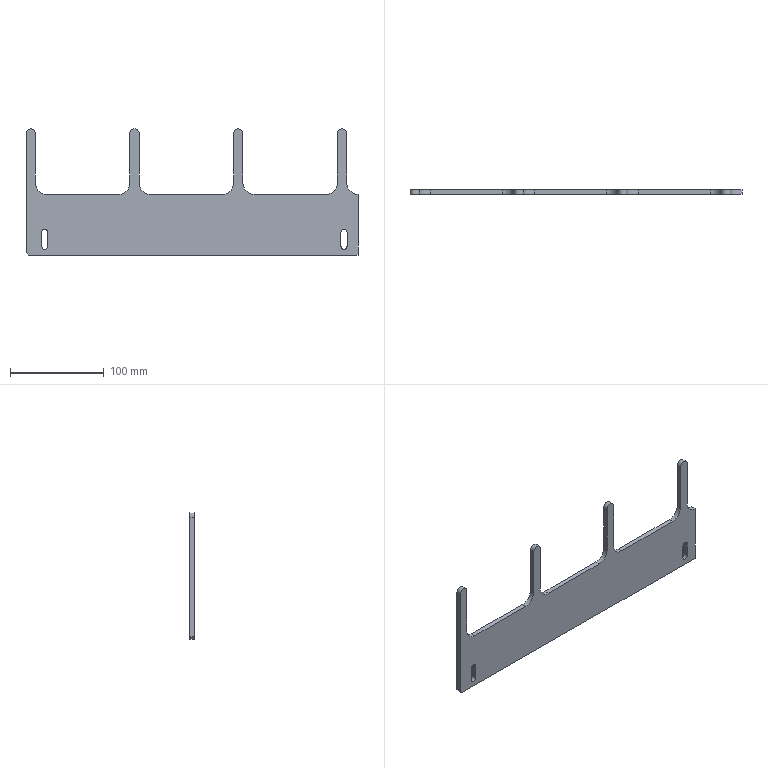Part | SolidWorks | features BaseBody 1, ICE 1 | 1 solid | 35 faces | box 355 x 5 x 135 mm | volume 128920 mm3 | plane 20 | cylinder 15 | commonest cylinder face diameters 24 x7 6.5 x4 10 x4
STEP:
#1=CARTESIAN_POINT('',(-205.,0.,-5.));
#2=VERTEX_POINT('',#1);
#3=CARTESIAN_POINT('',(-205.,0.,60.));
#4=VERTEX_POINT('',#3);
#5=CARTESIAN_POINT('',(-205.,0.,62.5));
#6=DIRECTION('',(0.,0.,1.));
#7=VECTOR('',#6,1000.);
#8=LINE('',#5,#7);
#9=EDGE_CURVE('',#2,#4,#8,.T.);
#10=ORIENTED_EDGE('',*,*,#9,.F.);
#11=CARTESIAN_POINT('',(-557.5,0.,-5.));
#12=VERTEX_POINT('',#11);
#13=CARTESIAN_POINT('',(-557.5,0.,-5.));
#14=DIRECTION('',(1.,0.,0.));
#15=VECTOR('',#14,1000.);
#16=LINE('',#13,#15);
#17=EDGE_CURVE('',#12,#2,#16,.T.);
#18=ORIENTED_EDGE('',*,*,#17,.F.);
#19=CARTESIAN_POINT('',(-560.,0.,-2.5));
#20=VERTEX_POINT('',#19);
#21=CARTESIAN_POINT('',(-560.,0.,-2.5));
#22=DIRECTION('',(0.7071,0.,-0.7071));
#23=VECTOR('',#22,1000.);
#24=LINE('',#21,#23);
#25=EDGE_CURVE('',#20,#12,#24,.T.);
#26=ORIENTED_EDGE('',*,*,#25,.F.);
#27=CARTESIAN_POINT('',(-560.,0.,125.));
#28=VERTEX_POINT('',#27);
#29=CARTESIAN_POINT('',(-560.,0.,125.));
#30=DIRECTION('',(0.,0.,-1.));
#31=VECTOR('',#30,1000.);
#32=LINE('',#29,#31);
#33=EDGE_CURVE('',#28,#20,#32,.T.);
#34=ORIENTED_EDGE('',*,*,#33,.F.);
#35=CARTESIAN_POINT('',(-550.,0.,125.));
#36=VERTEX_POINT('',#35);
#37=CARTESIAN_POINT('',(-555.,0.,125.));
#38=DIRECTION('',(0.,-1.,0.));
#39=DIRECTION('',(1.,0.,0.));
#40=AXIS2_PLACEMENT_3D('',#37,#38,#39);
#41=CIRCLE('',#40,5.);
#42=EDGE_CURVE('',#36,#28,#41,.T.);
#43=ORIENTED_EDGE('',*,*,#42,.F.);
#44=CARTESIAN_POINT('',(-550.,0.,72.));
#45=VERTEX_POINT('',#44);
#46=CARTESIAN_POINT('',(-550.,0.,72.));
#47=DIRECTION('',(0.,0.,1.));
#48=VECTOR('',#47,1000.);
#49=LINE('',#46,#48);
#50=EDGE_CURVE('',#45,#36,#49,.T.);
#51=ORIENTED_EDGE('',*,*,#50,.F.);
#52=CARTESIAN_POINT('',(-538.,0.,60.));
#53=VERTEX_POINT('',#52);
#54=CARTESIAN_POINT('',(-538.,0.,72.));
#55=DIRECTION('',(0.,1.,0.));
#56=DIRECTION('',(0.,0.,-1.));
#57=AXIS2_PLACEMENT_3D('',#54,#55,#56);
#58=CIRCLE('',#57,12.);
#59=EDGE_CURVE('',#53,#45,#58,.T.);
#60=ORIENTED_EDGE('',*,*,#59,.F.);
#61=CARTESIAN_POINT('',(-461.,0.,60.));
#62=VERTEX_POINT('',#61);
#63=CARTESIAN_POINT('',(-461.,0.,60.));
#64=DIRECTION('',(-1.,0.,0.));
#65=VECTOR('',#64,1000.);
#66=LINE('',#63,#65);
#67=EDGE_CURVE('',#62,#53,#66,.T.);
#68=ORIENTED_EDGE('',*,*,#67,.F.);
#69=CARTESIAN_POINT('',(-449.,0.,72.));
#70=VERTEX_POINT('',#69);
#71=CARTESIAN_POINT('',(-461.,0.,72.));
#72=DIRECTION('',(0.,1.,0.));
#73=DIRECTION('',(1.,0.,0.));
#74=AXIS2_PLACEMENT_3D('',#71,#72,#73);
#75=CIRCLE('',#74,12.);
#76=EDGE_CURVE('',#70,#62,#75,.T.);
#77=ORIENTED_EDGE('',*,*,#76,.F.);
#78=CARTESIAN_POINT('',(-449.,0.,125.));
#79=VERTEX_POINT('',#78);
#80=CARTESIAN_POINT('',(-449.,0.,125.));
#81=DIRECTION('',(0.,0.,-1.));
#82=VECTOR('',#81,1000.);
#83=LINE('',#80,#82);
#84=EDGE_CURVE('',#79,#70,#83,.T.);
#85=ORIENTED_EDGE('',*,*,#84,.F.);
#86=CARTESIAN_POINT('',(-439.,0.,125.));
#87=VERTEX_POINT('',#86);
#88=CARTESIAN_POINT('',(-444.,0.,125.));
#89=DIRECTION('',(0.,-1.,0.));
#90=DIRECTION('',(1.,0.,0.));
#91=AXIS2_PLACEMENT_3D('',#88,#89,#90);
#92=CIRCLE('',#91,5.);
#93=EDGE_CURVE('',#87,#79,#92,.T.);
#94=ORIENTED_EDGE('',*,*,#93,.F.);
#95=CARTESIAN_POINT('',(-439.,0.,72.));
#96=VERTEX_POINT('',#95);
#97=CARTESIAN_POINT('',(-439.,0.,72.));
#98=DIRECTION('',(0.,0.,1.));
#99=VECTOR('',#98,1000.);
#100=LINE('',#97,#99);
#101=EDGE_CURVE('',#96,#87,#100,.T.);
#102=ORIENTED_EDGE('',*,*,#101,.F.);
#103=CARTESIAN_POINT('',(-427.,0.,60.));
#104=VERTEX_POINT('',#103);
#105=CARTESIAN_POINT('',(-427.,0.,72.));
#106=DIRECTION('',(0.,1.,0.));
#107=DIRECTION('',(0.,0.,-1.));
#108=AXIS2_PLACEMENT_3D('',#105,#106,#107);
#109=CIRCLE('',#108,12.);
#110=EDGE_CURVE('',#104,#96,#109,.T.);
#111=ORIENTED_EDGE('',*,*,#110,.F.);
#112=CARTESIAN_POINT('',(-350.,0.,60.));
#113=VERTEX_POINT('',#112);
#114=CARTESIAN_POINT('',(-350.,0.,60.));
#115=DIRECTION('',(-1.,0.,0.));
#116=VECTOR('',#115,1000.);
#117=LINE('',#114,#116);
#118=EDGE_CURVE('',#113,#104,#117,.T.);
#119=ORIENTED_EDGE('',*,*,#118,.F.);
#120=CARTESIAN_POINT('',(-338.,0.,72.));
#121=VERTEX_POINT('',#120);
#122=CARTESIAN_POINT('',(-350.,0.,72.));
#123=DIRECTION('',(0.,1.,0.));
#124=DIRECTION('',(1.,0.,0.));
#125=AXIS2_PLACEMENT_3D('',#122,#123,#124);
#126=CIRCLE('',#125,12.);
#127=EDGE_CURVE('',#121,#113,#126,.T.);
#128=ORIENTED_EDGE('',*,*,#127,.F.);
#129=CARTESIAN_POINT('',(-338.,0.,125.));
#130=VERTEX_POINT('',#129);
#131=CARTESIAN_POINT('',(-338.,0.,125.));
#132=DIRECTION('',(0.,0.,-1.));
#133=VECTOR('',#132,1000.);
#134=LINE('',#131,#133);
#135=EDGE_CURVE('',#130,#121,#134,.T.);
#136=ORIENTED_EDGE('',*,*,#135,.F.);
#137=CARTESIAN_POINT('',(-328.,0.,125.));
#138=VERTEX_POINT('',#137);
#139=CARTESIAN_POINT('',(-333.,0.,125.));
#140=DIRECTION('',(0.,-1.,0.));
#141=DIRECTION('',(1.,0.,0.));
#142=AXIS2_PLACEMENT_3D('',#139,#140,#141);
#143=CIRCLE('',#142,5.);
#144=EDGE_CURVE('',#138,#130,#143,.T.);
#145=ORIENTED_EDGE('',*,*,#144,.F.);
#146=CARTESIAN_POINT('',(-328.,0.,72.));
#147=VERTEX_POINT('',#146);
#148=CARTESIAN_POINT('',(-328.,0.,72.));
#149=DIRECTION('',(0.,0.,1.));
#150=VECTOR('',#149,1000.);
#151=LINE('',#148,#150);
#152=EDGE_CURVE('',#147,#138,#151,.T.);
#153=ORIENTED_EDGE('',*,*,#152,.F.);
#154=CARTESIAN_POINT('',(-316.,0.,60.));
#155=VERTEX_POINT('',#154);
#156=CARTESIAN_POINT('',(-316.,0.,72.));
#157=DIRECTION('',(0.,1.,0.));
#158=DIRECTION('',(0.,0.,-1.));
#159=AXIS2_PLACEMENT_3D('',#156,#157,#158);
#160=CIRCLE('',#159,12.);
#161=EDGE_CURVE('',#155,#147,#160,.T.);
#162=ORIENTED_EDGE('',*,*,#161,.F.);
#163=CARTESIAN_POINT('',(-239.,0.,60.));
#164=VERTEX_POINT('',#163);
#165=CARTESIAN_POINT('',(-239.,0.,60.));
#166=DIRECTION('',(-1.,0.,0.));
#167=VECTOR('',#166,1000.);
#168=LINE('',#165,#167);
#169=EDGE_CURVE('',#164,#155,#168,.T.);
#170=ORIENTED_EDGE('',*,*,#169,.F.);
#171=CARTESIAN_POINT('',(-227.,0.,72.));
#172=VERTEX_POINT('',#171);
#173=CARTESIAN_POINT('',(-239.,0.,72.));
#174=DIRECTION('',(0.,1.,0.));
#175=DIRECTION('',(1.,0.,0.));
#176=AXIS2_PLACEMENT_3D('',#173,#174,#175);
#177=CIRCLE('',#176,12.);
#178=EDGE_CURVE('',#172,#164,#177,.T.);
#179=ORIENTED_EDGE('',*,*,#178,.F.);
#180=CARTESIAN_POINT('',(-227.,0.,125.));
#181=VERTEX_POINT('',#180);
#182=CARTESIAN_POINT('',(-227.,0.,125.));
#183=DIRECTION('',(0.,0.,-1.));
#184=VECTOR('',#183,1000.);
#185=LINE('',#182,#184);
#186=EDGE_CURVE('',#181,#172,#185,.T.);
#187=ORIENTED_EDGE('',*,*,#186,.F.);
#188=CARTESIAN_POINT('',(-217.,0.,125.));
#189=VERTEX_POINT('',#188);
#190=CARTESIAN_POINT('',(-222.,0.,125.));
#191=DIRECTION('',(0.,-1.,0.));
#192=DIRECTION('',(1.,0.,0.));
#193=AXIS2_PLACEMENT_3D('',#190,#191,#192);
#194=CIRCLE('',#193,5.);
#195=EDGE_CURVE('',#189,#181,#194,.T.);
#196=ORIENTED_EDGE('',*,*,#195,.F.);
#197=CARTESIAN_POINT('',(-217.,0.,72.));
#198=VERTEX_POINT('',#197);
#199=CARTESIAN_POINT('',(-217.,0.,72.));
#200=DIRECTION('',(0.,0.,1.));
#201=VECTOR('',#200,1000.);
#202=LINE('',#199,#201);
#203=EDGE_CURVE('',#198,#189,#202,.T.);
#204=ORIENTED_EDGE('',*,*,#203,.F.);
#205=CARTESIAN_POINT('',(-205.,0.,72.));
#206=DIRECTION('',(0.,1.,0.));
#207=DIRECTION('',(0.,0.,-1.));
#208=AXIS2_PLACEMENT_3D('',#205,#206,#207);
#209=CIRCLE('',#208,12.);
#210=EDGE_CURVE('',#4,#198,#209,.T.);
#211=ORIENTED_EDGE('',*,*,#210,.F.);
#212=EDGE_LOOP('',(#10,#18,#26,#34,#43,#51,#60,#68,#77,#85,#94,#102,#111,#119,#128,#136,#145,#153,#162,#170,#179,#187,#196,#204,#211));
#213=FACE_OUTER_BOUND('',#212,.T.);
#214=CARTESIAN_POINT('',(-536.75,0.,4.5));
#215=VERTEX_POINT('',#214);
#216=CARTESIAN_POINT('',(-543.25,0.,4.5));
#217=VERTEX_POINT('',#216);
#218=CARTESIAN_POINT('',(-540.,0.,4.5));
#219=DIRECTION('',(0.,1.,0.));
#220=DIRECTION('',(1.,0.,0.));
#221=AXIS2_PLACEMENT_3D('',#218,#219,#220);
#222=CIRCLE('',#221,3.25);
#223=EDGE_CURVE('',#215,#217,#222,.T.);
#224=ORIENTED_EDGE('',*,*,#223,.F.);
#225=CARTESIAN_POINT('',(-536.75,0.,19.5));
#226=VERTEX_POINT('',#225);
#227=CARTESIAN_POINT('',(-536.75,0.,19.5));
#228=DIRECTION('',(0.,0.,-1.));
#229=VECTOR('',#228,1000.);
#230=LINE('',#227,#229);
#231=EDGE_CURVE('',#226,#215,#230,.T.);
#232=ORIENTED_EDGE('',*,*,#231,.F.);
#233=CARTESIAN_POINT('',(-543.25,0.,19.5));
#234=VERTEX_POINT('',#233);
#235=CARTESIAN_POINT('',(-540.,0.,19.5));
#236=DIRECTION('',(0.,1.,0.));
#237=DIRECTION('',(-1.,0.,0.));
#238=AXIS2_PLACEMENT_3D('',#235,#236,#237);
#239=CIRCLE('',#238,3.25);
#240=EDGE_CURVE('',#234,#226,#239,.T.);
#241=ORIENTED_EDGE('',*,*,#240,.F.);
#242=CARTESIAN_POINT('',(-543.25,0.,4.5));
#243=DIRECTION('',(0.,0.,1.));
#244=VECTOR('',#243,1000.);
#245=LINE('',#242,#244);
#246=EDGE_CURVE('',#217,#234,#245,.T.);
#247=ORIENTED_EDGE('',*,*,#246,.F.);
#248=EDGE_LOOP('',(#224,#232,#241,#247));
#249=FACE_BOUND('',#248,.T.);
#250=CARTESIAN_POINT('',(-216.75,0.,4.5));
#251=VERTEX_POINT('',#250);
#252=CARTESIAN_POINT('',(-223.25,0.,4.5));
#253=VERTEX_POINT('',#252);
#254=CARTESIAN_POINT('',(-220.,0.,4.5));
#255=DIRECTION('',(0.,1.,0.));
#256=DIRECTION('',(1.,0.,0.));
#257=AXIS2_PLACEMENT_3D('',#254,#255,#256);
#258=CIRCLE('',#257,3.25);
#259=EDGE_CURVE('',#251,#253,#258,.T.);
#260=ORIENTED_EDGE('',*,*,#259,.F.);
#261=CARTESIAN_POINT('',(-216.75,0.,19.5));
#262=VERTEX_POINT('',#261);
#263=CARTESIAN_POINT('',(-216.75,0.,19.5));
#264=DIRECTION('',(0.,0.,-1.));
#265=VECTOR('',#264,1000.);
#266=LINE('',#263,#265);
#267=EDGE_CURVE('',#262,#251,#266,.T.);
#268=ORIENTED_EDGE('',*,*,#267,.F.);
#269=CARTESIAN_POINT('',(-223.25,0.,19.5));
#270=VERTEX_POINT('',#269);
#271=CARTESIAN_POINT('',(-220.,0.,19.5));
#272=DIRECTION('',(0.,1.,0.));
#273=DIRECTION('',(-1.,0.,0.));
#274=AXIS2_PLACEMENT_3D('',#271,#272,#273);
#275=CIRCLE('',#274,3.25);
#276=EDGE_CURVE('',#270,#262,#275,.T.);
#277=ORIENTED_EDGE('',*,*,#276,.F.);
#278=CARTESIAN_POINT('',(-223.25,0.,4.5));
#279=DIRECTION('',(0.,0.,1.));
#280=VECTOR('',#279,1000.);
#281=LINE('',#278,#280);
#282=EDGE_CURVE('',#253,#270,#281,.T.);
#283=ORIENTED_EDGE('',*,*,#282,.F.);
#284=EDGE_LOOP('',(#260,#268,#277,#283));
#285=FACE_BOUND('',#284,.T.);
#286=CARTESIAN_POINT('',(0.,0.,62.5));
#287=DIRECTION('',(0.,1.,0.));
#288=DIRECTION('',(0.,0.,-1.));
#289=AXIS2_PLACEMENT_3D('',#286,#287,#288);
#290=PLANE('',#289);
#291=ADVANCED_FACE('',(#213,#249,#285),#290,.T.);
#292=CARTESIAN_POINT('',(-205.,-5.,60.));
#293=VERTEX_POINT('',#292);
#294=CARTESIAN_POINT('',(-205.,-5.,-5.));
#295=VERTEX_POINT('',#294);
#296=CARTESIAN_POINT('',(-205.,-5.,60.));
#297=DIRECTION('',(0.,0.,-1.));
#298=VECTOR('',#297,1000.);
#299=LINE('',#296,#298);
#300=EDGE_CURVE('',#293,#295,#299,.T.);
#301=ORIENTED_EDGE('',*,*,#300,.F.);
#302=CARTESIAN_POINT('',(-217.,-5.,72.));
#303=VERTEX_POINT('',#302);
#304=CARTESIAN_POINT('',(-205.,-5.,72.));
#305=DIRECTION('',(0.,-1.,0.));
#306=DIRECTION('',(-1.,0.,0.));
#307=AXIS2_PLACEMENT_3D('',#304,#305,#306);
#308=CIRCLE('',#307,12.);
#309=EDGE_CURVE('',#303,#293,#308,.T.);
#310=ORIENTED_EDGE('',*,*,#309,.F.);
#311=CARTESIAN_POINT('',(-217.,-5.,125.));
#312=VERTEX_POINT('',#311);
#313=CARTESIAN_POINT('',(-217.,-5.,125.));
#314=DIRECTION('',(0.,0.,-1.));
#315=VECTOR('',#314,1000.);
#316=LINE('',#313,#315);
#317=EDGE_CURVE('',#312,#303,#316,.T.);
#318=ORIENTED_EDGE('',*,*,#317,.F.);
#319=CARTESIAN_POINT('',(-227.,-5.,125.));
#320=VERTEX_POINT('',#319);
#321=CARTESIAN_POINT('',(-222.,-5.,125.));
#322=DIRECTION('',(0.,1.,0.));
#323=DIRECTION('',(-1.,0.,0.));
#324=AXIS2_PLACEMENT_3D('',#321,#322,#323);
#325=CIRCLE('',#324,5.);
#326=EDGE_CURVE('',#320,#312,#325,.T.);
#327=ORIENTED_EDGE('',*,*,#326,.F.);
#328=CARTESIAN_POINT('',(-227.,-5.,72.));
#329=VERTEX_POINT('',#328);
#330=CARTESIAN_POINT('',(-227.,-5.,72.));
#331=DIRECTION('',(0.,0.,1.));
#332=VECTOR('',#331,1000.);
#333=LINE('',#330,#332);
#334=EDGE_CURVE('',#329,#320,#333,.T.);
#335=ORIENTED_EDGE('',*,*,#334,.F.);
#336=CARTESIAN_POINT('',(-239.,-5.,60.));
#337=VERTEX_POINT('',#336);
#338=CARTESIAN_POINT('',(-239.,-5.,72.));
#339=DIRECTION('',(0.,-1.,0.));
#340=DIRECTION('',(0.,0.,-1.));
#341=AXIS2_PLACEMENT_3D('',#338,#339,#340);
#342=CIRCLE('',#341,12.);
#343=EDGE_CURVE('',#337,#329,#342,.T.);
#344=ORIENTED_EDGE('',*,*,#343,.F.);
#345=CARTESIAN_POINT('',(-316.,-5.,60.));
#346=VERTEX_POINT('',#345);
#347=CARTESIAN_POINT('',(-316.,-5.,60.));
#348=DIRECTION('',(1.,0.,0.));
#349=VECTOR('',#348,1000.);
#350=LINE('',#347,#349);
#351=EDGE_CURVE('',#346,#337,#350,.T.);
#352=ORIENTED_EDGE('',*,*,#351,.F.);
#353=CARTESIAN_POINT('',(-328.,-5.,72.));
#354=VERTEX_POINT('',#353);
#355=CARTESIAN_POINT('',(-316.,-5.,72.));
#356=DIRECTION('',(0.,-1.,0.));
#357=DIRECTION('',(-1.,0.,0.));
#358=AXIS2_PLACEMENT_3D('',#355,#356,#357);
#359=CIRCLE('',#358,12.);
#360=EDGE_CURVE('',#354,#346,#359,.T.);
#361=ORIENTED_EDGE('',*,*,#360,.F.);
#362=CARTESIAN_POINT('',(-328.,-5.,125.));
#363=VERTEX_POINT('',#362);
#364=CARTESIAN_POINT('',(-328.,-5.,125.));
#365=DIRECTION('',(0.,0.,-1.));
#366=VECTOR('',#365,1000.);
#367=LINE('',#364,#366);
#368=EDGE_CURVE('',#363,#354,#367,.T.);
#369=ORIENTED_EDGE('',*,*,#368,.F.);
#370=CARTESIAN_POINT('',(-338.,-5.,125.));
#371=VERTEX_POINT('',#370);
#372=CARTESIAN_POINT('',(-333.,-5.,125.));
#373=DIRECTION('',(0.,1.,0.));
#374=DIRECTION('',(-1.,0.,0.));
#375=AXIS2_PLACEMENT_3D('',#372,#373,#374);
#376=CIRCLE('',#375,5.);
#377=EDGE_CURVE('',#371,#363,#376,.T.);
#378=ORIENTED_EDGE('',*,*,#377,.F.);
#379=CARTESIAN_POINT('',(-338.,-5.,72.));
#380=VERTEX_POINT('',#379);
#381=CARTESIAN_POINT('',(-338.,-5.,72.));
#382=DIRECTION('',(0.,0.,1.));
#383=VECTOR('',#382,1000.);
#384=LINE('',#381,#383);
#385=EDGE_CURVE('',#380,#371,#384,.T.);
#386=ORIENTED_EDGE('',*,*,#385,.F.);
#387=CARTESIAN_POINT('',(-350.,-5.,60.));
#388=VERTEX_POINT('',#387);
#389=CARTESIAN_POINT('',(-350.,-5.,72.));
#390=DIRECTION('',(0.,-1.,0.));
#391=DIRECTION('',(0.,0.,-1.));
#392=AXIS2_PLACEMENT_3D('',#389,#390,#391);
#393=CIRCLE('',#392,12.);
#394=EDGE_CURVE('',#388,#380,#393,.T.);
#395=ORIENTED_EDGE('',*,*,#394,.F.);
#396=CARTESIAN_POINT('',(-427.,-5.,60.));
#397=VERTEX_POINT('',#396);
#398=CARTESIAN_POINT('',(-427.,-5.,60.));
#399=DIRECTION('',(1.,0.,0.));
#400=VECTOR('',#399,1000.);
#401=LINE('',#398,#400);
#402=EDGE_CURVE('',#397,#388,#401,.T.);
#403=ORIENTED_EDGE('',*,*,#402,.F.);
#404=CARTESIAN_POINT('',(-439.,-5.,72.));
#405=VERTEX_POINT('',#404);
#406=CARTESIAN_POINT('',(-427.,-5.,72.));
#407=DIRECTION('',(0.,-1.,0.));
#408=DIRECTION('',(-1.,0.,0.));
#409=AXIS2_PLACEMENT_3D('',#406,#407,#408);
#410=CIRCLE('',#409,12.);
#411=EDGE_CURVE('',#405,#397,#410,.T.);
#412=ORIENTED_EDGE('',*,*,#411,.F.);
#413=CARTESIAN_POINT('',(-439.,-5.,125.));
#414=VERTEX_POINT('',#413);
#415=CARTESIAN_POINT('',(-439.,-5.,125.));
#416=DIRECTION('',(0.,0.,-1.));
#417=VECTOR('',#416,1000.);
#418=LINE('',#415,#417);
#419=EDGE_CURVE('',#414,#405,#418,.T.);
#420=ORIENTED_EDGE('',*,*,#419,.F.);
#421=CARTESIAN_POINT('',(-449.,-5.,125.));
#422=VERTEX_POINT('',#421);
#423=CARTESIAN_POINT('',(-444.,-5.,125.));
#424=DIRECTION('',(0.,1.,0.));
#425=DIRECTION('',(-1.,0.,0.));
#426=AXIS2_PLACEMENT_3D('',#423,#424,#425);
#427=CIRCLE('',#426,5.);
#428=EDGE_CURVE('',#422,#414,#427,.T.);
#429=ORIENTED_EDGE('',*,*,#428,.F.);
#430=CARTESIAN_POINT('',(-449.,-5.,72.));
#431=VERTEX_POINT('',#430);
#432=CARTESIAN_POINT('',(-449.,-5.,72.));
#433=DIRECTION('',(0.,0.,1.));
#434=VECTOR('',#433,1000.);
#435=LINE('',#432,#434);
#436=EDGE_CURVE('',#431,#422,#435,.T.);
#437=ORIENTED_EDGE('',*,*,#436,.F.);
#438=CARTESIAN_POINT('',(-461.,-5.,60.));
#439=VERTEX_POINT('',#438);
#440=CARTESIAN_POINT('',(-461.,-5.,72.));
#441=DIRECTION('',(0.,-1.,0.));
#442=DIRECTION('',(0.,0.,-1.));
#443=AXIS2_PLACEMENT_3D('',#440,#441,#442);
#444=CIRCLE('',#443,12.);
#445=EDGE_CURVE('',#439,#431,#444,.T.);
#446=ORIENTED_EDGE('',*,*,#445,.F.);
#447=CARTESIAN_POINT('',(-538.,-5.,60.));
#448=VERTEX_POINT('',#447);
#449=CARTESIAN_POINT('',(-538.,-5.,60.));
#450=DIRECTION('',(1.,0.,0.));
#451=VECTOR('',#450,1000.);
#452=LINE('',#449,#451);
#453=EDGE_CURVE('',#448,#439,#452,.T.);
#454=ORIENTED_EDGE('',*,*,#453,.F.);
#455=CARTESIAN_POINT('',(-550.,-5.,72.));
#456=VERTEX_POINT('',#455);
#457=CARTESIAN_POINT('',(-538.,-5.,72.));
#458=DIRECTION('',(0.,-1.,0.));
#459=DIRECTION('',(-1.,0.,0.));
#460=AXIS2_PLACEMENT_3D('',#457,#458,#459);
#461=CIRCLE('',#460,12.);
#462=EDGE_CURVE('',#456,#448,#461,.T.);
#463=ORIENTED_EDGE('',*,*,#462,.F.);
#464=CARTESIAN_POINT('',(-550.,-5.,125.));
#465=VERTEX_POINT('',#464);
#466=CARTESIAN_POINT('',(-550.,-5.,125.));
#467=DIRECTION('',(0.,0.,-1.));
#468=VECTOR('',#467,1000.);
#469=LINE('',#466,#468);
#470=EDGE_CURVE('',#465,#456,#469,.T.);
#471=ORIENTED_EDGE('',*,*,#470,.F.);
#472=CARTESIAN_POINT('',(-560.,-5.,125.));
#473=VERTEX_POINT('',#472);
#474=CARTESIAN_POINT('',(-555.,-5.,125.));
#475=DIRECTION('',(0.,1.,0.));
#476=DIRECTION('',(-1.,0.,0.));
#477=AXIS2_PLACEMENT_3D('',#474,#475,#476);
#478=CIRCLE('',#477,5.);
#479=EDGE_CURVE('',#473,#465,#478,.T.);
#480=ORIENTED_EDGE('',*,*,#479,.F.);
#481=CARTESIAN_POINT('',(-560.,-5.,-2.5));
#482=VERTEX_POINT('',#481);
#483=CARTESIAN_POINT('',(-560.,-5.,-2.5));
#484=DIRECTION('',(0.,0.,1.));
#485=VECTOR('',#484,1000.);
#486=LINE('',#483,#485);
#487=EDGE_CURVE('',#482,#473,#486,.T.);
#488=ORIENTED_EDGE('',*,*,#487,.F.);
#489=CARTESIAN_POINT('',(-557.5,-5.,-5.));
#490=VERTEX_POINT('',#489);
#491=CARTESIAN_POINT('',(-557.5,-5.,-5.));
#492=DIRECTION('',(-0.7071,0.,0.7071));
#493=VECTOR('',#492,1000.);
#494=LINE('',#491,#493);
#495=EDGE_CURVE('',#490,#482,#494,.T.);
#496=ORIENTED_EDGE('',*,*,#495,.F.);
#497=CARTESIAN_POINT('',(557.5,-5.,-5.));
#498=DIRECTION('',(-1.,0.,0.));
#499=VECTOR('',#498,1000.);
#500=LINE('',#497,#499);
#501=EDGE_CURVE('',#295,#490,#500,.T.);
#502=ORIENTED_EDGE('',*,*,#501,.F.);
#503=EDGE_LOOP('',(#301,#310,#318,#327,#335,#344,#352,#361,#369,#378,#386,#395,#403,#412,#420,#429,#437,#446,#454,#463,#471,#480,#488,#496,#502));
#504=FACE_OUTER_BOUND('',#503,.T.);
#505=CARTESIAN_POINT('',(-543.25,-5.,4.5));
#506=VERTEX_POINT('',#505);
#507=CARTESIAN_POINT('',(-536.75,-5.,4.5));
#508=VERTEX_POINT('',#507);
#509=CARTESIAN_POINT('',(-540.,-5.,4.5));
#510=DIRECTION('',(0.,-1.,0.));
#511=DIRECTION('',(-1.,0.,0.));
#512=AXIS2_PLACEMENT_3D('',#509,#510,#511);
#513=CIRCLE('',#512,3.25);
#514=EDGE_CURVE('',#506,#508,#513,.T.);
#515=ORIENTED_EDGE('',*,*,#514,.F.);
#516=CARTESIAN_POINT('',(-543.25,-5.,19.5));
#517=VERTEX_POINT('',#516);
#518=CARTESIAN_POINT('',(-543.25,-5.,19.5));
#519=DIRECTION('',(0.,0.,-1.));
#520=VECTOR('',#519,1000.);
#521=LINE('',#518,#520);
#522=EDGE_CURVE('',#517,#506,#521,.T.);
#523=ORIENTED_EDGE('',*,*,#522,.F.);
#524=CARTESIAN_POINT('',(-536.75,-5.,19.5));
#525=VERTEX_POINT('',#524);
#526=CARTESIAN_POINT('',(-540.,-5.,19.5));
#527=DIRECTION('',(0.,-1.,0.));
#528=DIRECTION('',(1.,0.,0.));
#529=AXIS2_PLACEMENT_3D('',#526,#527,#528);
#530=CIRCLE('',#529,3.25);
#531=EDGE_CURVE('',#525,#517,#530,.T.);
#532=ORIENTED_EDGE('',*,*,#531,.F.);
#533=CARTESIAN_POINT('',(-536.75,-5.,4.5));
#534=DIRECTION('',(0.,0.,1.));
#535=VECTOR('',#534,1000.);
#536=LINE('',#533,#535);
#537=EDGE_CURVE('',#508,#525,#536,.T.);
#538=ORIENTED_EDGE('',*,*,#537,.F.);
#539=EDGE_LOOP('',(#515,#523,#532,#538));
#540=FACE_BOUND('',#539,.T.);
#541=CARTESIAN_POINT('',(-223.25,-5.,4.5));
#542=VERTEX_POINT('',#541);
#543=CARTESIAN_POINT('',(-216.75,-5.,4.5));
#544=VERTEX_POINT('',#543);
#545=CARTESIAN_POINT('',(-220.,-5.,4.5));
#546=DIRECTION('',(0.,-1.,0.));
#547=DIRECTION('',(-1.,0.,0.));
#548=AXIS2_PLACEMENT_3D('',#545,#546,#547);
#549=CIRCLE('',#548,3.25);
#550=EDGE_CURVE('',#542,#544,#549,.T.);
#551=ORIENTED_EDGE('',*,*,#550,.F.);
#552=CARTESIAN_POINT('',(-223.25,-5.,19.5));
#553=VERTEX_POINT('',#552);
#554=CARTESIAN_POINT('',(-223.25,-5.,19.5));
#555=DIRECTION('',(0.,0.,-1.));
#556=VECTOR('',#555,1000.);
#557=LINE('',#554,#556);
#558=EDGE_CURVE('',#553,#542,#557,.T.);
#559=ORIENTED_EDGE('',*,*,#558,.F.);
#560=CARTESIAN_POINT('',(-216.75,-5.,19.5));
#561=VERTEX_POINT('',#560);
#562=CARTESIAN_POINT('',(-220.,-5.,19.5));
#563=DIRECTION('',(0.,-1.,0.));
#564=DIRECTION('',(1.,0.,0.));
#565=AXIS2_PLACEMENT_3D('',#562,#563,#564);
#566=CIRCLE('',#565,3.25);
#567=EDGE_CURVE('',#561,#553,#566,.T.);
#568=ORIENTED_EDGE('',*,*,#567,.F.);
#569=CARTESIAN_POINT('',(-216.75,-5.,4.5));
#570=DIRECTION('',(0.,0.,1.));
#571=VECTOR('',#570,1000.);
#572=LINE('',#569,#571);
#573=EDGE_CURVE('',#544,#561,#572,.T.);
#574=ORIENTED_EDGE('',*,*,#573,.F.);
#575=EDGE_LOOP('',(#551,#559,#568,#574));
#576=FACE_BOUND('',#575,.T.);
#577=CARTESIAN_POINT('',(0.,-5.,62.5));
#578=DIRECTION('',(0.,-1.,0.));
#579=DIRECTION('',(0.,0.,-1.));
#580=AXIS2_PLACEMENT_3D('',#577,#578,#579);
#581=PLANE('',#580);
#582=ADVANCED_FACE('',(#504,#540,#576),#581,.T.);
#583=ORIENTED_EDGE('',*,*,#210,.T.);
#584=CARTESIAN_POINT('',(-217.,-5.,72.));
#585=DIRECTION('',(0.,1.,0.));
#586=VECTOR('',#585,1000.);
#587=LINE('',#584,#586);
#588=EDGE_CURVE('',#303,#198,#587,.T.);
#589=ORIENTED_EDGE('',*,*,#588,.F.);
#590=ORIENTED_EDGE('',*,*,#309,.T.);
#591=CARTESIAN_POINT('',(-205.,-5.,60.));
#592=DIRECTION('',(0.,1.,0.));
#593=VECTOR('',#592,1000.);
#594=LINE('',#591,#593);
#595=EDGE_CURVE('',#293,#4,#594,.T.);
#596=ORIENTED_EDGE('',*,*,#595,.T.);
#597=EDGE_LOOP('',(#583,#589,#590,#596));
#598=FACE_OUTER_BOUND('',#597,.T.);
#599=CARTESIAN_POINT('',(-205.,0.,72.));
#600=DIRECTION('',(0.,-1.,0.));
#601=DIRECTION('',(-1.,0.,0.000005163));
#602=AXIS2_PLACEMENT_3D('',#599,#600,#601);
#603=CYLINDRICAL_SURFACE('',#602,12.);
#604=ADVANCED_FACE('',(#598),#603,.F.);
#605=ORIENTED_EDGE('',*,*,#203,.T.);
#606=CARTESIAN_POINT('',(-217.,-5.,125.));
#607=DIRECTION('',(0.,1.,0.));
#608=VECTOR('',#607,1000.);
#609=LINE('',#606,#608);
#610=EDGE_CURVE('',#312,#189,#609,.T.);
#611=ORIENTED_EDGE('',*,*,#610,.F.);
#612=ORIENTED_EDGE('',*,*,#317,.T.);
#613=ORIENTED_EDGE('',*,*,#588,.T.);
#614=EDGE_LOOP('',(#605,#611,#612,#613));
#615=FACE_OUTER_BOUND('',#614,.T.);
#616=CARTESIAN_POINT('',(-217.,0.,72.));
#617=DIRECTION('',(1.,0.,0.));
#618=DIRECTION('',(0.,1.,0.));
#619=AXIS2_PLACEMENT_3D('',#616,#617,#618);
#620=PLANE('',#619);
#621=ADVANCED_FACE('',(#615),#620,.T.);
#622=ORIENTED_EDGE('',*,*,#195,.T.);
#623=CARTESIAN_POINT('',(-227.,-5.,125.));
#624=DIRECTION('',(0.,1.,0.));
#625=VECTOR('',#624,1000.);
#626=LINE('',#623,#625);
#627=EDGE_CURVE('',#320,#181,#626,.T.);
#628=ORIENTED_EDGE('',*,*,#627,.F.);
#629=ORIENTED_EDGE('',*,*,#326,.T.);
#630=ORIENTED_EDGE('',*,*,#610,.T.);
#631=EDGE_LOOP('',(#622,#628,#629,#630));
#632=FACE_OUTER_BOUND('',#631,.T.);
#633=CARTESIAN_POINT('',(-222.,0.,125.));
#634=DIRECTION('',(0.,-1.,0.));
#635=DIRECTION('',(-1.,0.,0.));
#636=AXIS2_PLACEMENT_3D('',#633,#634,#635);
#637=CYLINDRICAL_SURFACE('',#636,5.);
#638=ADVANCED_FACE('',(#632),#637,.T.);
#639=ORIENTED_EDGE('',*,*,#186,.T.);
#640=CARTESIAN_POINT('',(-227.,-5.,72.));
#641=DIRECTION('',(0.,1.,0.));
#642=VECTOR('',#641,1000.);
#643=LINE('',#640,#642);
#644=EDGE_CURVE('',#329,#172,#643,.T.);
#645=ORIENTED_EDGE('',*,*,#644,.F.);
#646=ORIENTED_EDGE('',*,*,#334,.T.);
#647=ORIENTED_EDGE('',*,*,#627,.T.);
#648=EDGE_LOOP('',(#639,#645,#646,#647));
#649=FACE_OUTER_BOUND('',#648,.T.);
#650=CARTESIAN_POINT('',(-227.,0.,125.));
#651=DIRECTION('',(-1.,0.,0.));
#652=DIRECTION('',(0.,0.,1.));
#653=AXIS2_PLACEMENT_3D('',#650,#651,#652);
#654=PLANE('',#653);
#655=ADVANCED_FACE('',(#649),#654,.T.);
#656=ORIENTED_EDGE('',*,*,#178,.T.);
#657=CARTESIAN_POINT('',(-239.,-5.,60.));
#658=DIRECTION('',(0.,1.,0.));
#659=VECTOR('',#658,1000.);
#660=LINE('',#657,#659);
#661=EDGE_CURVE('',#337,#164,#660,.T.);
#662=ORIENTED_EDGE('',*,*,#661,.F.);
#663=ORIENTED_EDGE('',*,*,#343,.T.);
#664=ORIENTED_EDGE('',*,*,#644,.T.);
#665=EDGE_LOOP('',(#656,#662,#663,#664));
#666=FACE_OUTER_BOUND('',#665,.T.);
#667=CARTESIAN_POINT('',(-239.,0.,72.));
#668=DIRECTION('',(0.,-1.,0.));
#669=DIRECTION('',(-0.000005112,0.,-1.));
#670=AXIS2_PLACEMENT_3D('',#667,#668,#669);
#671=CYLINDRICAL_SURFACE('',#670,12.);
#672=ADVANCED_FACE('',(#666),#671,.F.);
#673=ORIENTED_EDGE('',*,*,#169,.T.);
#674=CARTESIAN_POINT('',(-316.,-5.,60.));
#675=DIRECTION('',(0.,1.,0.));
#676=VECTOR('',#675,1000.);
#677=LINE('',#674,#676);
#678=EDGE_CURVE('',#346,#155,#677,.T.);
#679=ORIENTED_EDGE('',*,*,#678,.F.);
#680=ORIENTED_EDGE('',*,*,#351,.T.);
#681=ORIENTED_EDGE('',*,*,#661,.T.);
#682=EDGE_LOOP('',(#673,#679,#680,#681));
#683=FACE_OUTER_BOUND('',#682,.T.);
#684=CARTESIAN_POINT('',(-239.,0.,60.));
#685=DIRECTION('',(0.,0.,1.));
#686=DIRECTION('',(1.,0.,0.));
#687=AXIS2_PLACEMENT_3D('',#684,#685,#686);
#688=PLANE('',#687);
#689=ADVANCED_FACE('',(#683),#688,.T.);
#690=ORIENTED_EDGE('',*,*,#161,.T.);
#691=CARTESIAN_POINT('',(-328.,-5.,72.));
#692=DIRECTION('',(0.,1.,0.));
#693=VECTOR('',#692,1000.);
#694=LINE('',#691,#693);
#695=EDGE_CURVE('',#354,#147,#694,.T.);
#696=ORIENTED_EDGE('',*,*,#695,.F.);
#697=ORIENTED_EDGE('',*,*,#360,.T.);
#698=ORIENTED_EDGE('',*,*,#678,.T.);
#699=EDGE_LOOP('',(#690,#696,#697,#698));
#700=FACE_OUTER_BOUND('',#699,.T.);
#701=CARTESIAN_POINT('',(-316.,0.,72.));
#702=DIRECTION('',(0.,-1.,0.));
#703=DIRECTION('',(-1.,0.,0.000005163));
#704=AXIS2_PLACEMENT_3D('',#701,#702,#703);
#705=CYLINDRICAL_SURFACE('',#704,12.);
#706=ADVANCED_FACE('',(#700),#705,.F.);
#707=ORIENTED_EDGE('',*,*,#152,.T.);
#708=CARTESIAN_POINT('',(-328.,-5.,125.));
#709=DIRECTION('',(0.,1.,0.));
#710=VECTOR('',#709,1000.);
#711=LINE('',#708,#710);
#712=EDGE_CURVE('',#363,#138,#711,.T.);
#713=ORIENTED_EDGE('',*,*,#712,.F.);
#714=ORIENTED_EDGE('',*,*,#368,.T.);
#715=ORIENTED_EDGE('',*,*,#695,.T.);
#716=EDGE_LOOP('',(#707,#713,#714,#715));
#717=FACE_OUTER_BOUND('',#716,.T.);
#718=CARTESIAN_POINT('',(-328.,0.,72.));
#719=DIRECTION('',(1.,0.,0.));
#720=DIRECTION('',(0.,1.,0.));
#721=AXIS2_PLACEMENT_3D('',#718,#719,#720);
#722=PLANE('',#721);
#723=ADVANCED_FACE('',(#717),#722,.T.);
#724=ORIENTED_EDGE('',*,*,#144,.T.);
#725=CARTESIAN_POINT('',(-338.,-5.,125.));
#726=DIRECTION('',(0.,1.,0.));
#727=VECTOR('',#726,1000.);
#728=LINE('',#725,#727);
#729=EDGE_CURVE('',#371,#130,#728,.T.);
#730=ORIENTED_EDGE('',*,*,#729,.F.);
#731=ORIENTED_EDGE('',*,*,#377,.T.);
#732=ORIENTED_EDGE('',*,*,#712,.T.);
#733=EDGE_LOOP('',(#724,#730,#731,#732));
#734=FACE_OUTER_BOUND('',#733,.T.);
#735=CARTESIAN_POINT('',(-333.,0.,125.));
#736=DIRECTION('',(0.,-1.,0.));
#737=DIRECTION('',(-1.,0.,0.));
#738=AXIS2_PLACEMENT_3D('',#735,#736,#737);
#739=CYLINDRICAL_SURFACE('',#738,5.);
#740=ADVANCED_FACE('',(#734),#739,.T.);
#741=ORIENTED_EDGE('',*,*,#135,.T.);
#742=CARTESIAN_POINT('',(-338.,-5.,72.));
#743=DIRECTION('',(0.,1.,0.));
#744=VECTOR('',#743,1000.);
#745=LINE('',#742,#744);
#746=EDGE_CURVE('',#380,#121,#745,.T.);
#747=ORIENTED_EDGE('',*,*,#746,.F.);
#748=ORIENTED_EDGE('',*,*,#385,.T.);
#749=ORIENTED_EDGE('',*,*,#729,.T.);
#750=EDGE_LOOP('',(#741,#747,#748,#749));
#751=FACE_OUTER_BOUND('',#750,.T.);
#752=CARTESIAN_POINT('',(-338.,0.,125.));
#753=DIRECTION('',(-1.,0.,0.));
#754=DIRECTION('',(0.,0.,1.));
#755=AXIS2_PLACEMENT_3D('',#752,#753,#754);
#756=PLANE('',#755);
#757=ADVANCED_FACE('',(#751),#756,.T.);
#758=ORIENTED_EDGE('',*,*,#127,.T.);
#759=CARTESIAN_POINT('',(-350.,-5.,60.));
#760=DIRECTION('',(0.,1.,0.));
#761=VECTOR('',#760,1000.);
#762=LINE('',#759,#761);
#763=EDGE_CURVE('',#388,#113,#762,.T.);
#764=ORIENTED_EDGE('',*,*,#763,.F.);
#765=ORIENTED_EDGE('',*,*,#394,.T.);
#766=ORIENTED_EDGE('',*,*,#746,.T.);
#767=EDGE_LOOP('',(#758,#764,#765,#766));
#768=FACE_OUTER_BOUND('',#767,.T.);
#769=CARTESIAN_POINT('',(-350.,0.,72.));
#770=DIRECTION('',(0.,-1.,0.));
#771=DIRECTION('',(-0.000005163,0.,-1.));
#772=AXIS2_PLACEMENT_3D('',#769,#770,#771);
#773=CYLINDRICAL_SURFACE('',#772,12.);
#774=ADVANCED_FACE('',(#768),#773,.F.);
#775=ORIENTED_EDGE('',*,*,#118,.T.);
#776=CARTESIAN_POINT('',(-427.,-5.,60.));
#777=DIRECTION('',(0.,1.,0.));
#778=VECTOR('',#777,1000.);
#779=LINE('',#776,#778);
#780=EDGE_CURVE('',#397,#104,#779,.T.);
#781=ORIENTED_EDGE('',*,*,#780,.F.);
#782=ORIENTED_EDGE('',*,*,#402,.T.);
#783=ORIENTED_EDGE('',*,*,#763,.T.);
#784=EDGE_LOOP('',(#775,#781,#782,#783));
#785=FACE_OUTER_BOUND('',#784,.T.);
#786=CARTESIAN_POINT('',(-350.,0.,60.));
#787=DIRECTION('',(0.,0.,1.));
#788=DIRECTION('',(1.,0.,0.));
#789=AXIS2_PLACEMENT_3D('',#786,#787,#788);
#790=PLANE('',#789);
#791=ADVANCED_FACE('',(#785),#790,.T.);
#792=ORIENTED_EDGE('',*,*,#110,.T.);
#793=CARTESIAN_POINT('',(-439.,-5.,72.));
#794=DIRECTION('',(0.,1.,0.));
#795=VECTOR('',#794,1000.);
#796=LINE('',#793,#795);
#797=EDGE_CURVE('',#405,#96,#796,.T.);
#798=ORIENTED_EDGE('',*,*,#797,.F.);
#799=ORIENTED_EDGE('',*,*,#411,.T.);
#800=ORIENTED_EDGE('',*,*,#780,.T.);
#801=EDGE_LOOP('',(#792,#798,#799,#800));
#802=FACE_OUTER_BOUND('',#801,.T.);
#803=CARTESIAN_POINT('',(-427.,0.,72.));
#804=DIRECTION('',(0.,-1.,0.));
#805=DIRECTION('',(-1.,0.,0.000005112));
#806=AXIS2_PLACEMENT_3D('',#803,#804,#805);
#807=CYLINDRICAL_SURFACE('',#806,12.);
#808=ADVANCED_FACE('',(#802),#807,.F.);
#809=ORIENTED_EDGE('',*,*,#101,.T.);
#810=CARTESIAN_POINT('',(-439.,-5.,125.));
#811=DIRECTION('',(0.,1.,0.));
#812=VECTOR('',#811,1000.);
#813=LINE('',#810,#812);
#814=EDGE_CURVE('',#414,#87,#813,.T.);
#815=ORIENTED_EDGE('',*,*,#814,.F.);
#816=ORIENTED_EDGE('',*,*,#419,.T.);
#817=ORIENTED_EDGE('',*,*,#797,.T.);
#818=EDGE_LOOP('',(#809,#815,#816,#817));
#819=FACE_OUTER_BOUND('',#818,.T.);
#820=CARTESIAN_POINT('',(-439.,0.,72.));
#821=DIRECTION('',(1.,0.,0.));
#822=DIRECTION('',(0.,1.,0.));
#823=AXIS2_PLACEMENT_3D('',#820,#821,#822);
#824=PLANE('',#823);
#825=ADVANCED_FACE('',(#819),#824,.T.);
#826=ORIENTED_EDGE('',*,*,#93,.T.);
#827=CARTESIAN_POINT('',(-449.,-5.,125.));
#828=DIRECTION('',(0.,1.,0.));
#829=VECTOR('',#828,1000.);
#830=LINE('',#827,#829);
#831=EDGE_CURVE('',#422,#79,#830,.T.);
#832=ORIENTED_EDGE('',*,*,#831,.F.);
#833=ORIENTED_EDGE('',*,*,#428,.T.);
#834=ORIENTED_EDGE('',*,*,#814,.T.);
#835=EDGE_LOOP('',(#826,#832,#833,#834));
#836=FACE_OUTER_BOUND('',#835,.T.);
#837=CARTESIAN_POINT('',(-444.,0.,125.));
#838=DIRECTION('',(0.,-1.,0.));
#839=DIRECTION('',(-1.,0.,0.));
#840=AXIS2_PLACEMENT_3D('',#837,#838,#839);
#841=CYLINDRICAL_SURFACE('',#840,5.);
#842=ADVANCED_FACE('',(#836),#841,.T.);
#843=ORIENTED_EDGE('',*,*,#84,.T.);
#844=CARTESIAN_POINT('',(-449.,-5.,72.));
#845=DIRECTION('',(0.,1.,0.));
#846=VECTOR('',#845,1000.);
#847=LINE('',#844,#846);
#848=EDGE_CURVE('',#431,#70,#847,.T.);
#849=ORIENTED_EDGE('',*,*,#848,.F.);
#850=ORIENTED_EDGE('',*,*,#436,.T.);
#851=ORIENTED_EDGE('',*,*,#831,.T.);
#852=EDGE_LOOP('',(#843,#849,#850,#851));
#853=FACE_OUTER_BOUND('',#852,.T.);
#854=CARTESIAN_POINT('',(-449.,0.,125.));
#855=DIRECTION('',(-1.,0.,0.));
#856=DIRECTION('',(0.,0.,1.));
#857=AXIS2_PLACEMENT_3D('',#854,#855,#856);
#858=PLANE('',#857);
#859=ADVANCED_FACE('',(#853),#858,.T.);
#860=ORIENTED_EDGE('',*,*,#76,.T.);
#861=CARTESIAN_POINT('',(-461.,-5.,60.));
#862=DIRECTION('',(0.,1.,0.));
#863=VECTOR('',#862,1000.);
#864=LINE('',#861,#863);
#865=EDGE_CURVE('',#439,#62,#864,.T.);
#866=ORIENTED_EDGE('',*,*,#865,.F.);
#867=ORIENTED_EDGE('',*,*,#445,.T.);
#868=ORIENTED_EDGE('',*,*,#848,.T.);
#869=EDGE_LOOP('',(#860,#866,#867,#868));
#870=FACE_OUTER_BOUND('',#869,.T.);
#871=CARTESIAN_POINT('',(-461.,0.,72.));
#872=DIRECTION('',(0.,-1.,0.));
#873=DIRECTION('',(-0.000005163,0.,-1.));
#874=AXIS2_PLACEMENT_3D('',#871,#872,#873);
#875=CYLINDRICAL_SURFACE('',#874,12.);
#876=ADVANCED_FACE('',(#870),#875,.F.);
#877=ORIENTED_EDGE('',*,*,#67,.T.);
#878=CARTESIAN_POINT('',(-538.,-5.,60.));
#879=DIRECTION('',(0.,1.,0.));
#880=VECTOR('',#879,1000.);
#881=LINE('',#878,#880);
#882=EDGE_CURVE('',#448,#53,#881,.T.);
#883=ORIENTED_EDGE('',*,*,#882,.F.);
#884=ORIENTED_EDGE('',*,*,#453,.T.);
#885=ORIENTED_EDGE('',*,*,#865,.T.);
#886=EDGE_LOOP('',(#877,#883,#884,#885));
#887=FACE_OUTER_BOUND('',#886,.T.);
#888=CARTESIAN_POINT('',(-461.,0.,60.));
#889=DIRECTION('',(0.,0.,1.));
#890=DIRECTION('',(0.,-1.,0.));
#891=AXIS2_PLACEMENT_3D('',#888,#889,#890);
#892=PLANE('',#891);
#893=ADVANCED_FACE('',(#887),#892,.T.);
#894=ORIENTED_EDGE('',*,*,#59,.T.);
#895=CARTESIAN_POINT('',(-550.,-5.,72.));
#896=DIRECTION('',(0.,1.,0.));
#897=VECTOR('',#896,1000.);
#898=LINE('',#895,#897);
#899=EDGE_CURVE('',#456,#45,#898,.T.);
#900=ORIENTED_EDGE('',*,*,#899,.F.);
#901=ORIENTED_EDGE('',*,*,#462,.T.);
#902=ORIENTED_EDGE('',*,*,#882,.T.);
#903=EDGE_LOOP('',(#894,#900,#901,#902));
#904=FACE_OUTER_BOUND('',#903,.T.);
#905=CARTESIAN_POINT('',(-538.,0.,72.));
#906=DIRECTION('',(0.,-1.,0.));
#907=DIRECTION('',(-1.,0.,0.000005163));
#908=AXIS2_PLACEMENT_3D('',#905,#906,#907);
#909=CYLINDRICAL_SURFACE('',#908,12.);
#910=ADVANCED_FACE('',(#904),#909,.F.);
#911=ORIENTED_EDGE('',*,*,#50,.T.);
#912=CARTESIAN_POINT('',(-550.,-5.,125.));
#913=DIRECTION('',(0.,1.,0.));
#914=VECTOR('',#913,1000.);
#915=LINE('',#912,#914);
#916=EDGE_CURVE('',#465,#36,#915,.T.);
#917=ORIENTED_EDGE('',*,*,#916,.F.);
#918=ORIENTED_EDGE('',*,*,#470,.T.);
#919=ORIENTED_EDGE('',*,*,#899,.T.);
#920=EDGE_LOOP('',(#911,#917,#918,#919));
#921=FACE_OUTER_BOUND('',#920,.T.);
#922=CARTESIAN_POINT('',(-550.,0.,72.));
#923=DIRECTION('',(1.,0.,0.));
#924=DIRECTION('',(0.,1.,0.));
#925=AXIS2_PLACEMENT_3D('',#922,#923,#924);
#926=PLANE('',#925);
#927=ADVANCED_FACE('',(#921),#926,.T.);
#928=ORIENTED_EDGE('',*,*,#42,.T.);
#929=CARTESIAN_POINT('',(-560.,-5.,125.));
#930=DIRECTION('',(0.,1.,0.));
#931=VECTOR('',#930,1000.);
#932=LINE('',#929,#931);
#933=EDGE_CURVE('',#473,#28,#932,.T.);
#934=ORIENTED_EDGE('',*,*,#933,.F.);
#935=ORIENTED_EDGE('',*,*,#479,.T.);
#936=ORIENTED_EDGE('',*,*,#916,.T.);
#937=EDGE_LOOP('',(#928,#934,#935,#936));
#938=FACE_OUTER_BOUND('',#937,.T.);
#939=CARTESIAN_POINT('',(-555.,0.,125.));
#940=DIRECTION('',(0.,-1.,0.));
#941=DIRECTION('',(-1.,0.,0.));
#942=AXIS2_PLACEMENT_3D('',#939,#940,#941);
#943=CYLINDRICAL_SURFACE('',#942,5.);
#944=ADVANCED_FACE('',(#938),#943,.T.);
#945=ORIENTED_EDGE('',*,*,#33,.T.);
#946=CARTESIAN_POINT('',(-560.,-5.,-2.5));
#947=DIRECTION('',(0.,1.,0.));
#948=VECTOR('',#947,1000.);
#949=LINE('',#946,#948);
#950=EDGE_CURVE('',#482,#20,#949,.T.);
#951=ORIENTED_EDGE('',*,*,#950,.F.);
#952=ORIENTED_EDGE('',*,*,#487,.T.);
#953=ORIENTED_EDGE('',*,*,#933,.T.);
#954=EDGE_LOOP('',(#945,#951,#952,#953));
#955=FACE_OUTER_BOUND('',#954,.T.);
#956=CARTESIAN_POINT('',(-560.,0.,125.));
#957=DIRECTION('',(-1.,0.,0.));
#958=DIRECTION('',(0.,0.,1.));
#959=AXIS2_PLACEMENT_3D('',#956,#957,#958);
#960=PLANE('',#959);
#961=ADVANCED_FACE('',(#955),#960,.T.);
#962=ORIENTED_EDGE('',*,*,#25,.T.);
#963=CARTESIAN_POINT('',(-557.5,-5.,-5.));
#964=DIRECTION('',(0.,1.,0.));
#965=VECTOR('',#964,1000.);
#966=LINE('',#963,#965);
#967=EDGE_CURVE('',#490,#12,#966,.T.);
#968=ORIENTED_EDGE('',*,*,#967,.F.);
#969=ORIENTED_EDGE('',*,*,#495,.T.);
#970=ORIENTED_EDGE('',*,*,#950,.T.);
#971=EDGE_LOOP('',(#962,#968,#969,#970));
#972=FACE_OUTER_BOUND('',#971,.T.);
#973=CARTESIAN_POINT('',(-560.,0.,-2.5));
#974=DIRECTION('',(-0.7071,0.,-0.7071));
#975=DIRECTION('',(-0.7071,0.,0.7071));
#976=AXIS2_PLACEMENT_3D('',#973,#974,#975);
#977=PLANE('',#976);
#978=ADVANCED_FACE('',(#972),#977,.T.);
#979=CARTESIAN_POINT('',(-205.,0.,-5.));
#980=DIRECTION('',(0.,1.,0.));
#981=VECTOR('',#980,1000.);
#982=LINE('',#979,#981);
#983=EDGE_CURVE('',#295,#2,#982,.T.);
#984=ORIENTED_EDGE('',*,*,#983,.F.);
#985=ORIENTED_EDGE('',*,*,#501,.T.);
#986=ORIENTED_EDGE('',*,*,#967,.T.);
#987=ORIENTED_EDGE('',*,*,#17,.T.);
#988=EDGE_LOOP('',(#984,#985,#986,#987));
#989=FACE_OUTER_BOUND('',#988,.T.);
#990=CARTESIAN_POINT('',(-557.5,0.,-5.));
#991=DIRECTION('',(0.,0.,-1.));
#992=DIRECTION('',(-1.,0.,0.));
#993=AXIS2_PLACEMENT_3D('',#990,#991,#992);
#994=PLANE('',#993);
#995=ADVANCED_FACE('',(#989),#994,.T.);
#996=ORIENTED_EDGE('',*,*,#223,.T.);
#997=CARTESIAN_POINT('',(-543.25,-5.,4.5));
#998=DIRECTION('',(0.,1.,0.));
#999=VECTOR('',#998,1000.);
#1000=LINE('',#997,#999);
#1001=EDGE_CURVE('',#506,#217,#1000,.T.);
#1002=ORIENTED_EDGE('',*,*,#1001,.F.);
#1003=ORIENTED_EDGE('',*,*,#514,.T.);
#1004=CARTESIAN_POINT('',(-536.75,0.,4.5));
#1005=DIRECTION('',(0.,-1.,0.));
#1006=VECTOR('',#1005,1000.);
#1007=LINE('',#1004,#1006);
#1008=EDGE_CURVE('',#215,#508,#1007,.T.);
#1009=ORIENTED_EDGE('',*,*,#1008,.F.);
#1010=EDGE_LOOP('',(#996,#1002,#1003,#1009));
#1011=FACE_OUTER_BOUND('',#1010,.T.);
#1012=CARTESIAN_POINT('',(-540.,0.,4.5));
#1013=DIRECTION('',(0.,-1.,0.));
#1014=DIRECTION('',(-1.,0.,0.));
#1015=AXIS2_PLACEMENT_3D('',#1012,#1013,#1014);
#1016=CYLINDRICAL_SURFACE('',#1015,3.25);
#1017=ADVANCED_FACE('',(#1011),#1016,.F.);
#1018=ORIENTED_EDGE('',*,*,#246,.T.);
#1019=CARTESIAN_POINT('',(-543.25,-5.,19.5));
#1020=DIRECTION('',(0.,1.,0.));
#1021=VECTOR('',#1020,1000.);
#1022=LINE('',#1019,#1021);
#1023=EDGE_CURVE('',#517,#234,#1022,.T.);
#1024=ORIENTED_EDGE('',*,*,#1023,.F.);
#1025=ORIENTED_EDGE('',*,*,#522,.T.);
#1026=ORIENTED_EDGE('',*,*,#1001,.T.);
#1027=EDGE_LOOP('',(#1018,#1024,#1025,#1026));
#1028=FACE_OUTER_BOUND('',#1027,.T.);
#1029=CARTESIAN_POINT('',(-543.25,0.,4.5));
#1030=DIRECTION('',(1.,0.,0.));
#1031=DIRECTION('',(0.,1.,0.));
#1032=AXIS2_PLACEMENT_3D('',#1029,#1030,#1031);
#1033=PLANE('',#1032);
#1034=ADVANCED_FACE('',(#1028),#1033,.T.);
#1035=ORIENTED_EDGE('',*,*,#240,.T.);
#1036=CARTESIAN_POINT('',(-536.75,-5.,19.5));
#1037=DIRECTION('',(0.,1.,0.));
#1038=VECTOR('',#1037,1000.);
#1039=LINE('',#1036,#1038);
#1040=EDGE_CURVE('',#525,#226,#1039,.T.);
#1041=ORIENTED_EDGE('',*,*,#1040,.F.);
#1042=ORIENTED_EDGE('',*,*,#531,.T.);
#1043=ORIENTED_EDGE('',*,*,#1023,.T.);
#1044=EDGE_LOOP('',(#1035,#1041,#1042,#1043));
#1045=FACE_OUTER_BOUND('',#1044,.T.);
#1046=CARTESIAN_POINT('',(-540.,0.,19.5));
#1047=DIRECTION('',(0.,-1.,0.));
#1048=DIRECTION('',(1.,0.,0.));
#1049=AXIS2_PLACEMENT_3D('',#1046,#1047,#1048);
#1050=CYLINDRICAL_SURFACE('',#1049,3.25);
#1051=ADVANCED_FACE('',(#1045),#1050,.F.);
#1052=ORIENTED_EDGE('',*,*,#231,.T.);
#1053=ORIENTED_EDGE('',*,*,#1008,.T.);
#1054=ORIENTED_EDGE('',*,*,#537,.T.);
#1055=ORIENTED_EDGE('',*,*,#1040,.T.);
#1056=EDGE_LOOP('',(#1052,#1053,#1054,#1055));
#1057=FACE_OUTER_BOUND('',#1056,.T.);
#1058=CARTESIAN_POINT('',(-536.75,0.,19.5));
#1059=DIRECTION('',(-1.,0.,0.));
#1060=DIRECTION('',(0.,0.,1.));
#1061=AXIS2_PLACEMENT_3D('',#1058,#1059,#1060);
#1062=PLANE('',#1061);
#1063=ADVANCED_FACE('',(#1057),#1062,.T.);
#1064=ORIENTED_EDGE('',*,*,#259,.T.);
#1065=CARTESIAN_POINT('',(-223.25,-5.,4.5));
#1066=DIRECTION('',(0.,1.,0.));
#1067=VECTOR('',#1066,1000.);
#1068=LINE('',#1065,#1067);
#1069=EDGE_CURVE('',#542,#253,#1068,.T.);
#1070=ORIENTED_EDGE('',*,*,#1069,.F.);
#1071=ORIENTED_EDGE('',*,*,#550,.T.);
#1072=CARTESIAN_POINT('',(-216.75,0.,4.5));
#1073=DIRECTION('',(0.,-1.,0.));
#1074=VECTOR('',#1073,1000.);
#1075=LINE('',#1072,#1074);
#1076=EDGE_CURVE('',#251,#544,#1075,.T.);
#1077=ORIENTED_EDGE('',*,*,#1076,.F.);
#1078=EDGE_LOOP('',(#1064,#1070,#1071,#1077));
#1079=FACE_OUTER_BOUND('',#1078,.T.);
#1080=CARTESIAN_POINT('',(-220.,0.,4.5));
#1081=DIRECTION('',(0.,-1.,0.));
#1082=DIRECTION('',(-1.,0.,0.));
#1083=AXIS2_PLACEMENT_3D('',#1080,#1081,#1082);
#1084=CYLINDRICAL_SURFACE('',#1083,3.25);
#1085=ADVANCED_FACE('',(#1079),#1084,.F.);
#1086=ORIENTED_EDGE('',*,*,#282,.T.);
#1087=CARTESIAN_POINT('',(-223.25,-5.,19.5));
#1088=DIRECTION('',(0.,1.,0.));
#1089=VECTOR('',#1088,1000.);
#1090=LINE('',#1087,#1089);
#1091=EDGE_CURVE('',#553,#270,#1090,.T.);
#1092=ORIENTED_EDGE('',*,*,#1091,.F.);
#1093=ORIENTED_EDGE('',*,*,#558,.T.);
#1094=ORIENTED_EDGE('',*,*,#1069,.T.);
#1095=EDGE_LOOP('',(#1086,#1092,#1093,#1094));
#1096=FACE_OUTER_BOUND('',#1095,.T.);
#1097=CARTESIAN_POINT('',(-223.25,0.,4.5));
#1098=DIRECTION('',(1.,0.,0.));
#1099=DIRECTION('',(0.,0.,1.));
#1100=AXIS2_PLACEMENT_3D('',#1097,#1098,#1099);
#1101=PLANE('',#1100);
#1102=ADVANCED_FACE('',(#1096),#1101,.T.);
#1103=ORIENTED_EDGE('',*,*,#276,.T.);
#1104=CARTESIAN_POINT('',(-216.75,-5.,19.5));
#1105=DIRECTION('',(0.,1.,0.));
#1106=VECTOR('',#1105,1000.);
#1107=LINE('',#1104,#1106);
#1108=EDGE_CURVE('',#561,#262,#1107,.T.);
#1109=ORIENTED_EDGE('',*,*,#1108,.F.);
#1110=ORIENTED_EDGE('',*,*,#567,.T.);
#1111=ORIENTED_EDGE('',*,*,#1091,.T.);
#1112=EDGE_LOOP('',(#1103,#1109,#1110,#1111));
#1113=FACE_OUTER_BOUND('',#1112,.T.);
#1114=CARTESIAN_POINT('',(-220.,0.,19.5));
#1115=DIRECTION('',(0.,-1.,0.));
#1116=DIRECTION('',(1.,0.,0.));
#1117=AXIS2_PLACEMENT_3D('',#1114,#1115,#1116);
#1118=CYLINDRICAL_SURFACE('',#1117,3.25);
#1119=ADVANCED_FACE('',(#1113),#1118,.F.);
#1120=ORIENTED_EDGE('',*,*,#267,.T.);
#1121=ORIENTED_EDGE('',*,*,#1076,.T.);
#1122=ORIENTED_EDGE('',*,*,#573,.T.);
#1123=ORIENTED_EDGE('',*,*,#1108,.T.);
#1124=EDGE_LOOP('',(#1120,#1121,#1122,#1123));
#1125=FACE_OUTER_BOUND('',#1124,.T.);
#1126=CARTESIAN_POINT('',(-216.75,0.,19.5));
#1127=DIRECTION('',(-1.,0.,0.));
#1128=DIRECTION('',(0.,1.,0.));
#1129=AXIS2_PLACEMENT_3D('',#1126,#1127,#1128);
#1130=PLANE('',#1129);
#1131=ADVANCED_FACE('',(#1125),#1130,.T.);
#1132=ORIENTED_EDGE('',*,*,#9,.T.);
#1133=ORIENTED_EDGE('',*,*,#595,.F.);
#1134=ORIENTED_EDGE('',*,*,#300,.T.);
#1135=ORIENTED_EDGE('',*,*,#983,.T.);
#1136=EDGE_LOOP('',(#1132,#1133,#1134,#1135));
#1137=FACE_OUTER_BOUND('',#1136,.T.);
#1138=CARTESIAN_POINT('',(-205.,65.,60.));
#1139=DIRECTION('',(-1.,0.,0.));
#1140=DIRECTION('',(0.,0.,1.));
#1141=AXIS2_PLACEMENT_3D('',#1138,#1139,#1140);
#1142=PLANE('',#1141);
#1143=ADVANCED_FACE('',(#1137),#1142,.F.);
#1144=CLOSED_SHELL('',(#291,#582,#604,#621,#638,#655,#672,#689,#706,#723,#740,#757,#774,#791,#808,#825,#842,#859,#876,#893,#910,#927,#944,#961,#978,#995,#1017,#1034,#1051,#1063,#1085,#1102,#1119,#1131,#1143));
#1145=MANIFOLD_SOLID_BREP('',#1144);
#1146=CARTESIAN_POINT('',(0.,0.,0.));
#1147=DIRECTION('',(0.,0.,1.));
#1148=DIRECTION('',(1.,0.,0.));
#1149=AXIS2_PLACEMENT_3D('',#1146,#1147,#1148);
#1150=(LENGTH_UNIT()NAMED_UNIT(*)SI_UNIT(.MILLI.,.METRE.));
#1151=UNCERTAINTY_MEASURE_WITH_UNIT(LENGTH_MEASURE(0.00001),#1150,'','');
#1152=(NAMED_UNIT(*)PLANE_ANGLE_UNIT()SI_UNIT($,.RADIAN.));
#1153=(NAMED_UNIT(*)SI_UNIT($,.STERADIAN.)SOLID_ANGLE_UNIT());
#1154=(GEOMETRIC_REPRESENTATION_CONTEXT(3)GLOBAL_UNCERTAINTY_ASSIGNED_CONTEXT((#1151))GLOBAL_UNIT_ASSIGNED_CONTEXT((#1150,#1152,#1153))REPRESENTATION_CONTEXT('',''));
#1155=ADVANCED_BREP_SHAPE_REPRESENTATION('',(#1145,#1149),#1154);